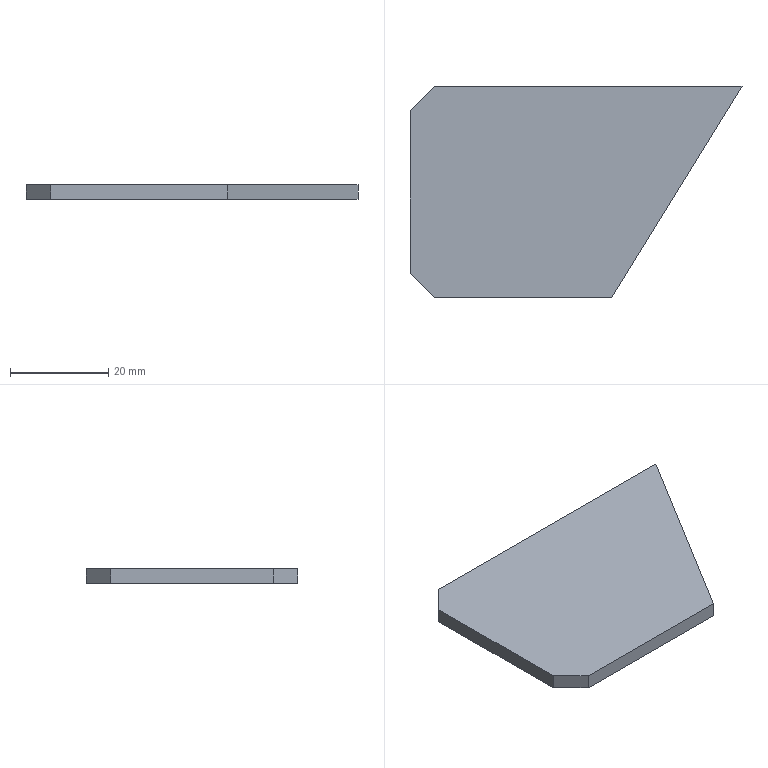Part | 1 solid | 8 faces | box 67.5 x 43 x 3 mm | volume 6923 mm3 | plane 8
STEP:
#1=CARTESIAN_POINT('',(67.5,21.5,-3.));
#2=VERTEX_POINT('',#1);
#3=CARTESIAN_POINT('',(5.,21.5,-3.));
#4=VERTEX_POINT('',#3);
#5=CARTESIAN_POINT('',(67.5,21.5,-3.));
#6=DIRECTION('',(-1.,0.,0.));
#7=VECTOR('',#6,1000.);
#8=LINE('',#5,#7);
#9=EDGE_CURVE('',#2,#4,#8,.T.);
#10=ORIENTED_EDGE('',*,*,#9,.T.);
#11=CARTESIAN_POINT('',(5.,21.5,0.));
#12=VERTEX_POINT('',#11);
#13=CARTESIAN_POINT('',(5.,21.5,-3.));
#14=DIRECTION('',(0.,0.,1.));
#15=VECTOR('',#14,1000.);
#16=LINE('',#13,#15);
#17=EDGE_CURVE('',#4,#12,#16,.T.);
#18=ORIENTED_EDGE('',*,*,#17,.T.);
#19=CARTESIAN_POINT('',(67.5,21.5,0.));
#20=VERTEX_POINT('',#19);
#21=CARTESIAN_POINT('',(67.5,21.5,0.));
#22=DIRECTION('',(-1.,0.,0.));
#23=VECTOR('',#22,1000.);
#24=LINE('',#21,#23);
#25=EDGE_CURVE('',#20,#12,#24,.T.);
#26=ORIENTED_EDGE('',*,*,#25,.F.);
#27=CARTESIAN_POINT('',(67.5,21.5,-3.));
#28=DIRECTION('',(0.,0.,1.));
#29=VECTOR('',#28,1000.);
#30=LINE('',#27,#29);
#31=EDGE_CURVE('',#2,#20,#30,.T.);
#32=ORIENTED_EDGE('',*,*,#31,.F.);
#33=EDGE_LOOP('',(#10,#18,#26,#32));
#34=FACE_OUTER_BOUND('',#33,.T.);
#35=CARTESIAN_POINT('',(67.5,21.5,-3.));
#36=DIRECTION('',(0.,1.,0.));
#37=DIRECTION('',(-1.,0.,0.));
#38=AXIS2_PLACEMENT_3D('',#35,#36,#37);
#39=PLANE('',#38);
#40=ADVANCED_FACE('',(#34),#39,.T.);
#41=CARTESIAN_POINT('',(41.,-21.5,0.));
#42=VERTEX_POINT('',#41);
#43=CARTESIAN_POINT('',(41.,-21.5,0.));
#44=DIRECTION('',(0.5246,0.8513,0.));
#45=VECTOR('',#44,1000.);
#46=LINE('',#43,#45);
#47=EDGE_CURVE('',#42,#20,#46,.T.);
#48=ORIENTED_EDGE('',*,*,#47,.F.);
#49=CARTESIAN_POINT('',(41.,-21.5,-3.));
#50=VERTEX_POINT('',#49);
#51=CARTESIAN_POINT('',(41.,-21.5,-3.));
#52=DIRECTION('',(0.,0.,1.));
#53=VECTOR('',#52,1000.);
#54=LINE('',#51,#53);
#55=EDGE_CURVE('',#50,#42,#54,.T.);
#56=ORIENTED_EDGE('',*,*,#55,.F.);
#57=CARTESIAN_POINT('',(41.,-21.5,-3.));
#58=DIRECTION('',(0.5246,0.8513,0.));
#59=VECTOR('',#58,1000.);
#60=LINE('',#57,#59);
#61=EDGE_CURVE('',#50,#2,#60,.T.);
#62=ORIENTED_EDGE('',*,*,#61,.T.);
#63=ORIENTED_EDGE('',*,*,#31,.T.);
#64=EDGE_LOOP('',(#48,#56,#62,#63));
#65=FACE_OUTER_BOUND('',#64,.T.);
#66=CARTESIAN_POINT('',(41.,-21.5,-3.));
#67=DIRECTION('',(0.8513,-0.5246,0.));
#68=DIRECTION('',(0.5246,0.8513,0.));
#69=AXIS2_PLACEMENT_3D('',#66,#67,#68);
#70=PLANE('',#69);
#71=ADVANCED_FACE('',(#65),#70,.T.);
#72=CARTESIAN_POINT('',(5.,-21.5,0.));
#73=VERTEX_POINT('',#72);
#74=CARTESIAN_POINT('',(0.,-21.5,0.));
#75=DIRECTION('',(1.,0.,0.));
#76=VECTOR('',#75,1000.);
#77=LINE('',#74,#76);
#78=EDGE_CURVE('',#73,#42,#77,.T.);
#79=ORIENTED_EDGE('',*,*,#78,.F.);
#80=CARTESIAN_POINT('',(5.,-21.5,-3.));
#81=VERTEX_POINT('',#80);
#82=CARTESIAN_POINT('',(5.,-21.5,-3.));
#83=DIRECTION('',(0.,0.,-1.));
#84=VECTOR('',#83,1000.);
#85=LINE('',#82,#84);
#86=EDGE_CURVE('',#73,#81,#85,.T.);
#87=ORIENTED_EDGE('',*,*,#86,.T.);
#88=CARTESIAN_POINT('',(0.,-21.5,-3.));
#89=DIRECTION('',(1.,0.,0.));
#90=VECTOR('',#89,1000.);
#91=LINE('',#88,#90);
#92=EDGE_CURVE('',#81,#50,#91,.T.);
#93=ORIENTED_EDGE('',*,*,#92,.T.);
#94=ORIENTED_EDGE('',*,*,#55,.T.);
#95=EDGE_LOOP('',(#79,#87,#93,#94));
#96=FACE_OUTER_BOUND('',#95,.T.);
#97=CARTESIAN_POINT('',(0.,-21.5,-3.));
#98=DIRECTION('',(0.,-1.,0.));
#99=DIRECTION('',(0.,0.,-1.));
#100=AXIS2_PLACEMENT_3D('',#97,#98,#99);
#101=PLANE('',#100);
#102=ADVANCED_FACE('',(#96),#101,.T.);
#103=CARTESIAN_POINT('',(0.,16.5,-3.));
#104=VERTEX_POINT('',#103);
#105=CARTESIAN_POINT('',(0.,-16.5,-3.));
#106=VERTEX_POINT('',#105);
#107=CARTESIAN_POINT('',(0.,21.5,-3.));
#108=DIRECTION('',(0.,-1.,0.));
#109=VECTOR('',#108,1000.);
#110=LINE('',#107,#109);
#111=EDGE_CURVE('',#104,#106,#110,.T.);
#112=ORIENTED_EDGE('',*,*,#111,.T.);
#113=CARTESIAN_POINT('',(0.,-16.5,0.));
#114=VERTEX_POINT('',#113);
#115=CARTESIAN_POINT('',(0.,-16.5,-3.));
#116=DIRECTION('',(0.,0.,1.));
#117=VECTOR('',#116,1000.);
#118=LINE('',#115,#117);
#119=EDGE_CURVE('',#106,#114,#118,.T.);
#120=ORIENTED_EDGE('',*,*,#119,.T.);
#121=CARTESIAN_POINT('',(0.,16.5,0.));
#122=VERTEX_POINT('',#121);
#123=CARTESIAN_POINT('',(0.,21.5,0.));
#124=DIRECTION('',(0.,-1.,0.));
#125=VECTOR('',#124,1000.);
#126=LINE('',#123,#125);
#127=EDGE_CURVE('',#122,#114,#126,.T.);
#128=ORIENTED_EDGE('',*,*,#127,.F.);
#129=CARTESIAN_POINT('',(0.,16.5,-3.));
#130=DIRECTION('',(0.,0.,-1.));
#131=VECTOR('',#130,1000.);
#132=LINE('',#129,#131);
#133=EDGE_CURVE('',#122,#104,#132,.T.);
#134=ORIENTED_EDGE('',*,*,#133,.T.);
#135=EDGE_LOOP('',(#112,#120,#128,#134));
#136=FACE_OUTER_BOUND('',#135,.T.);
#137=CARTESIAN_POINT('',(0.,21.5,-3.));
#138=DIRECTION('',(-1.,0.,0.));
#139=DIRECTION('',(0.,-1.,0.));
#140=AXIS2_PLACEMENT_3D('',#137,#138,#139);
#141=PLANE('',#140);
#142=ADVANCED_FACE('',(#136),#141,.T.);
#143=ORIENTED_EDGE('',*,*,#92,.F.);
#144=CARTESIAN_POINT('',(0.,-16.5,-3.));
#145=DIRECTION('',(-0.7071,0.7071,0.));
#146=VECTOR('',#145,1000.);
#147=LINE('',#144,#146);
#148=EDGE_CURVE('',#81,#106,#147,.T.);
#149=ORIENTED_EDGE('',*,*,#148,.T.);
#150=ORIENTED_EDGE('',*,*,#111,.F.);
#151=CARTESIAN_POINT('',(5.,21.5,-3.));
#152=DIRECTION('',(0.7071,0.7071,0.));
#153=VECTOR('',#152,1000.);
#154=LINE('',#151,#153);
#155=EDGE_CURVE('',#104,#4,#154,.T.);
#156=ORIENTED_EDGE('',*,*,#155,.T.);
#157=ORIENTED_EDGE('',*,*,#9,.F.);
#158=ORIENTED_EDGE('',*,*,#61,.F.);
#159=EDGE_LOOP('',(#143,#149,#150,#156,#157,#158));
#160=FACE_OUTER_BOUND('',#159,.T.);
#161=CARTESIAN_POINT('',(0.,0.,-3.));
#162=DIRECTION('',(0.,0.,1.));
#163=DIRECTION('',(1.,0.,0.));
#164=AXIS2_PLACEMENT_3D('',#161,#162,#163);
#165=PLANE('',#164);
#166=ADVANCED_FACE('',(#160),#165,.F.);
#167=ORIENTED_EDGE('',*,*,#127,.T.);
#168=CARTESIAN_POINT('',(-8.25,-8.25,0.));
#169=DIRECTION('',(0.7071,-0.7071,0.));
#170=VECTOR('',#169,1000.);
#171=LINE('',#168,#170);
#172=EDGE_CURVE('',#114,#73,#171,.T.);
#173=ORIENTED_EDGE('',*,*,#172,.T.);
#174=ORIENTED_EDGE('',*,*,#78,.T.);
#175=ORIENTED_EDGE('',*,*,#47,.T.);
#176=ORIENTED_EDGE('',*,*,#25,.T.);
#177=CARTESIAN_POINT('',(-8.25,8.25,0.));
#178=DIRECTION('',(-0.7071,-0.7071,0.));
#179=VECTOR('',#178,1000.);
#180=LINE('',#177,#179);
#181=EDGE_CURVE('',#12,#122,#180,.T.);
#182=ORIENTED_EDGE('',*,*,#181,.T.);
#183=EDGE_LOOP('',(#167,#173,#174,#175,#176,#182));
#184=FACE_OUTER_BOUND('',#183,.T.);
#185=CARTESIAN_POINT('',(0.,0.,0.));
#186=DIRECTION('',(0.,0.,1.));
#187=DIRECTION('',(1.,0.,0.));
#188=AXIS2_PLACEMENT_3D('',#185,#186,#187);
#189=PLANE('',#188);
#190=ADVANCED_FACE('',(#184),#189,.T.);
#191=ORIENTED_EDGE('',*,*,#148,.F.);
#192=ORIENTED_EDGE('',*,*,#86,.F.);
#193=ORIENTED_EDGE('',*,*,#172,.F.);
#194=ORIENTED_EDGE('',*,*,#119,.F.);
#195=EDGE_LOOP('',(#191,#192,#193,#194));
#196=FACE_OUTER_BOUND('',#195,.T.);
#197=CARTESIAN_POINT('',(0.,-16.5,-3.));
#198=DIRECTION('',(0.7071,0.7071,0.));
#199=DIRECTION('',(0.,0.,1.));
#200=AXIS2_PLACEMENT_3D('',#197,#198,#199);
#201=PLANE('',#200);
#202=ADVANCED_FACE('',(#196),#201,.F.);
#203=ORIENTED_EDGE('',*,*,#155,.F.);
#204=ORIENTED_EDGE('',*,*,#133,.F.);
#205=ORIENTED_EDGE('',*,*,#181,.F.);
#206=ORIENTED_EDGE('',*,*,#17,.F.);
#207=EDGE_LOOP('',(#203,#204,#205,#206));
#208=FACE_OUTER_BOUND('',#207,.T.);
#209=CARTESIAN_POINT('',(5.,21.5,-3.));
#210=DIRECTION('',(0.7071,-0.7071,0.));
#211=DIRECTION('',(0.,0.,1.));
#212=AXIS2_PLACEMENT_3D('',#209,#210,#211);
#213=PLANE('',#212);
#214=ADVANCED_FACE('',(#208),#213,.F.);
#215=CLOSED_SHELL('',(#40,#71,#102,#142,#166,#190,#202,#214));
#216=MANIFOLD_SOLID_BREP('',#215);
#217=CARTESIAN_POINT('',(0.,0.,0.));
#218=DIRECTION('',(0.,0.,1.));
#219=DIRECTION('',(1.,0.,0.));
#220=AXIS2_PLACEMENT_3D('',#217,#218,#219);
#221=(LENGTH_UNIT()NAMED_UNIT(*)SI_UNIT(.MILLI.,.METRE.));
#222=UNCERTAINTY_MEASURE_WITH_UNIT(LENGTH_MEASURE(0.00001),#221,'','');
#223=(NAMED_UNIT(*)PLANE_ANGLE_UNIT()SI_UNIT($,.RADIAN.));
#224=(NAMED_UNIT(*)SI_UNIT($,.STERADIAN.)SOLID_ANGLE_UNIT());
#225=(GEOMETRIC_REPRESENTATION_CONTEXT(3)GLOBAL_UNCERTAINTY_ASSIGNED_CONTEXT((#222))GLOBAL_UNIT_ASSIGNED_CONTEXT((#221,#223,#224))REPRESENTATION_CONTEXT('',''));
#226=ADVANCED_BREP_SHAPE_REPRESENTATION('',(#216,#220),#225);